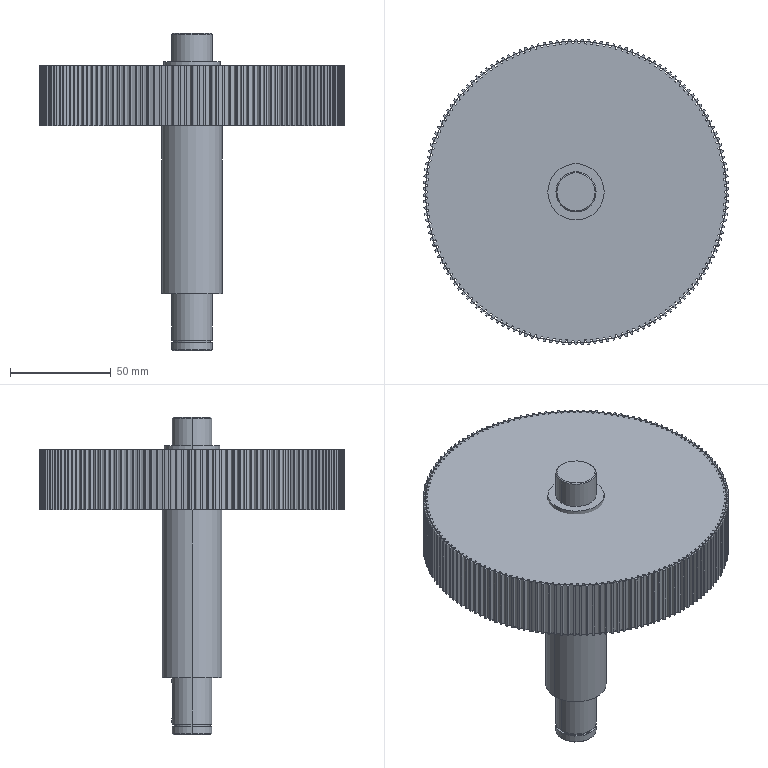Part | SolidWorks | 1 solid | 632 faces | box 151.981 x 152 x 157.8 mm | volume 267297 mm3 | cylinder 616 | plane 12 | cone 4 | commonest cylinder face diameters 29.932 x300 147.5 x150 152 x150 20 x6 6 x2 18.35 x2